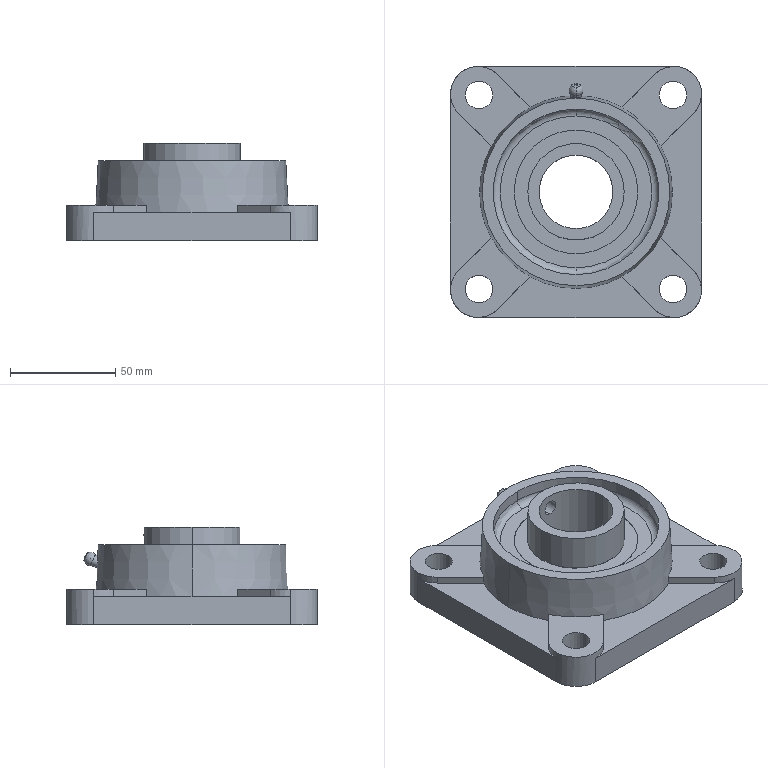Part | SolidWorks | features Revolution 5, Boss 2, RevCut 2, CirPattern 1, Cut 1, Extrusion 1 | 1 solid | 118 faces | box 119 x 119 x 46.4 mm | volume 215912 mm3 | cylinder 58 | plane 42 | sphere 10 | torus 6 | cone 2 | commonest cylinder face diameters 6 x14 26 x12 13 x8 45.73 x6 58.68 x6 78.48 x4